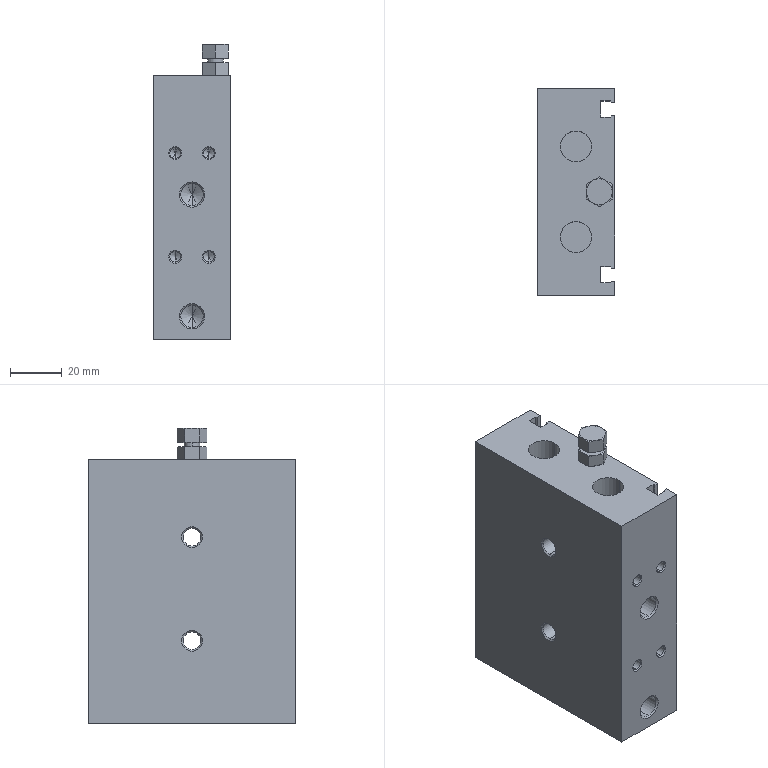Part | STEP file | CXSM25-30(0_0)_BODY_HI | 1 solid | 161 faces | box 30 x 80 x 114 mm | volume 192548 mm3 | cone 76 | plane 43 | cylinder 42 | commonest cylinder face diameters 4.134 x16 8.566 x8 6.9 x4 11 x4 12 x4 25 x4